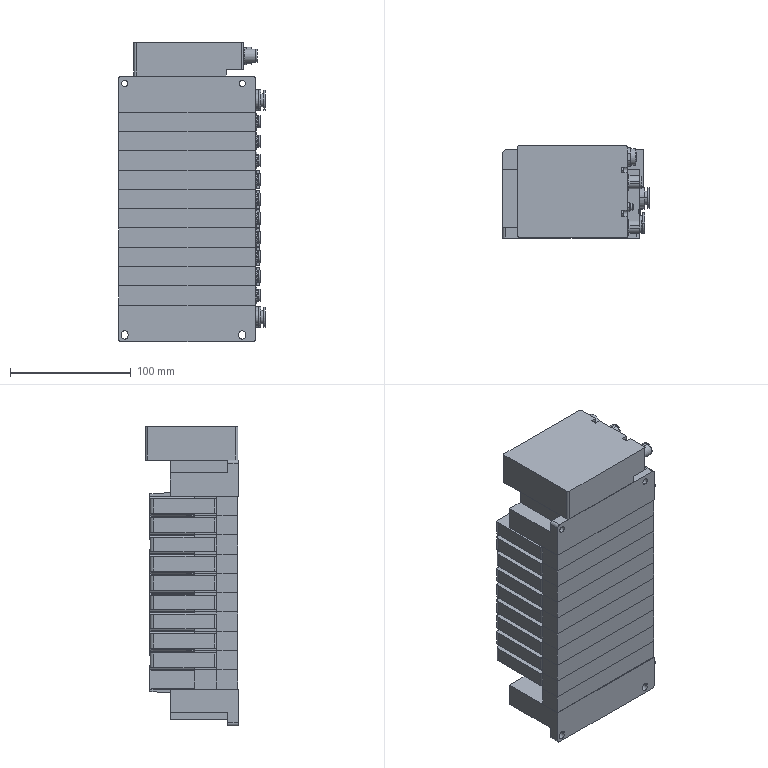Part | SolidWorks | 23 solids | 3737 faces | volume 1754450 mm3 | plane 2814 | cylinder 872 | spline 45 | cone 6 | commonest cylinder face diameters 6 x79 1.2 x54 5.5 x48 14 x48 10 x44 7.4 x40